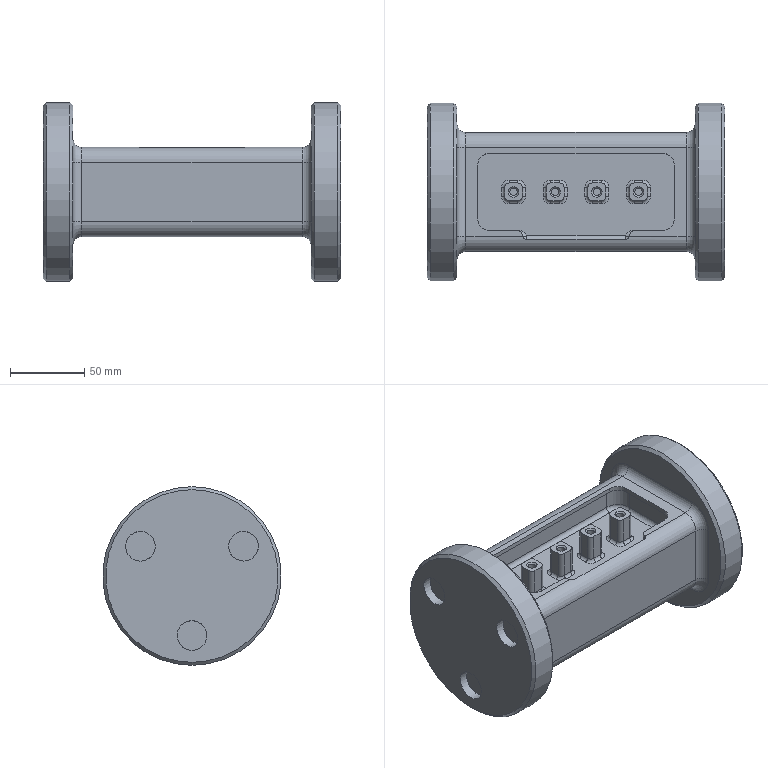Part | 1 solid | 167 faces | box 200 x 120 x 120 mm | volume 1047704 mm3 | cylinder 76 | plane 51 | torus 30 | cone 8 | sphere 2 | commonest cylinder face diameters 6 x28 4 x16 20 x10 12 x8 5 x4 16 x4